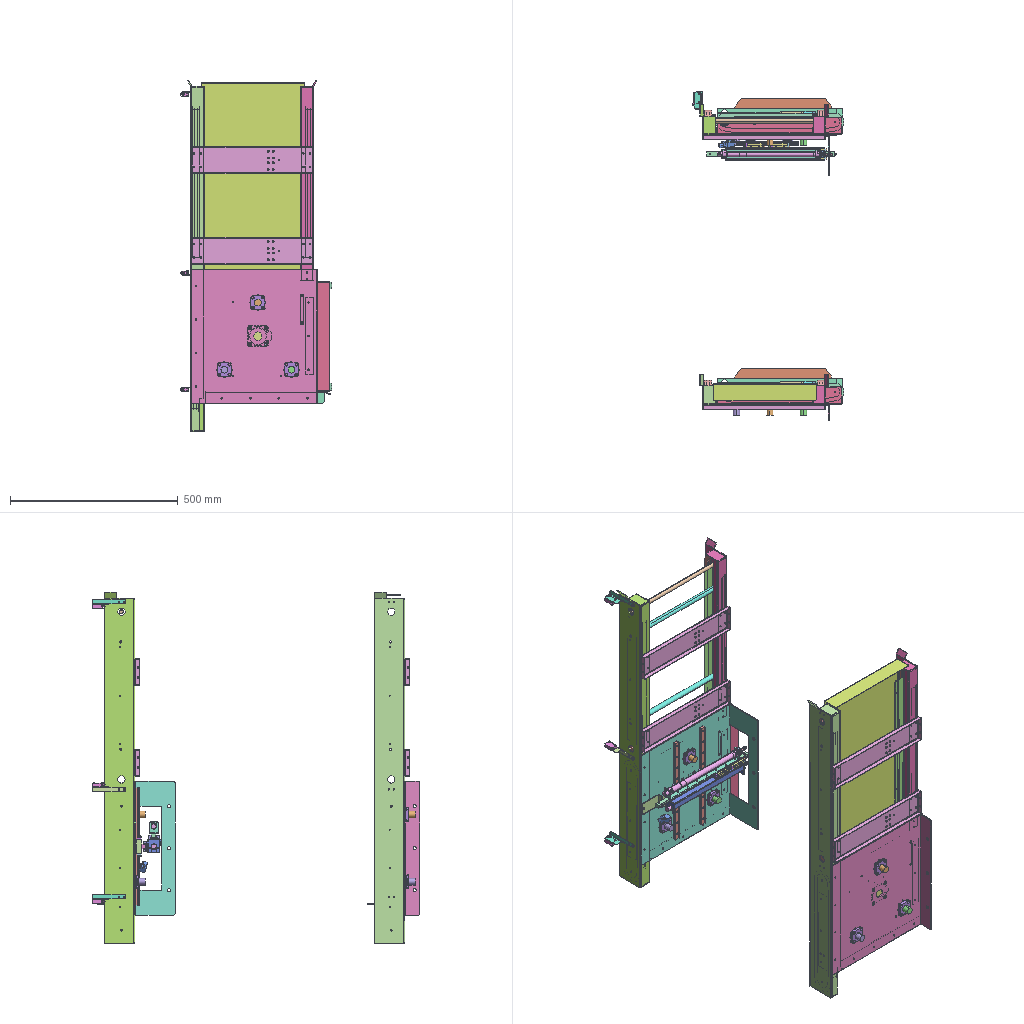Assembly | SolidWorks | 39 different items | 94 placed | box 453 x 977 x 1048 mm
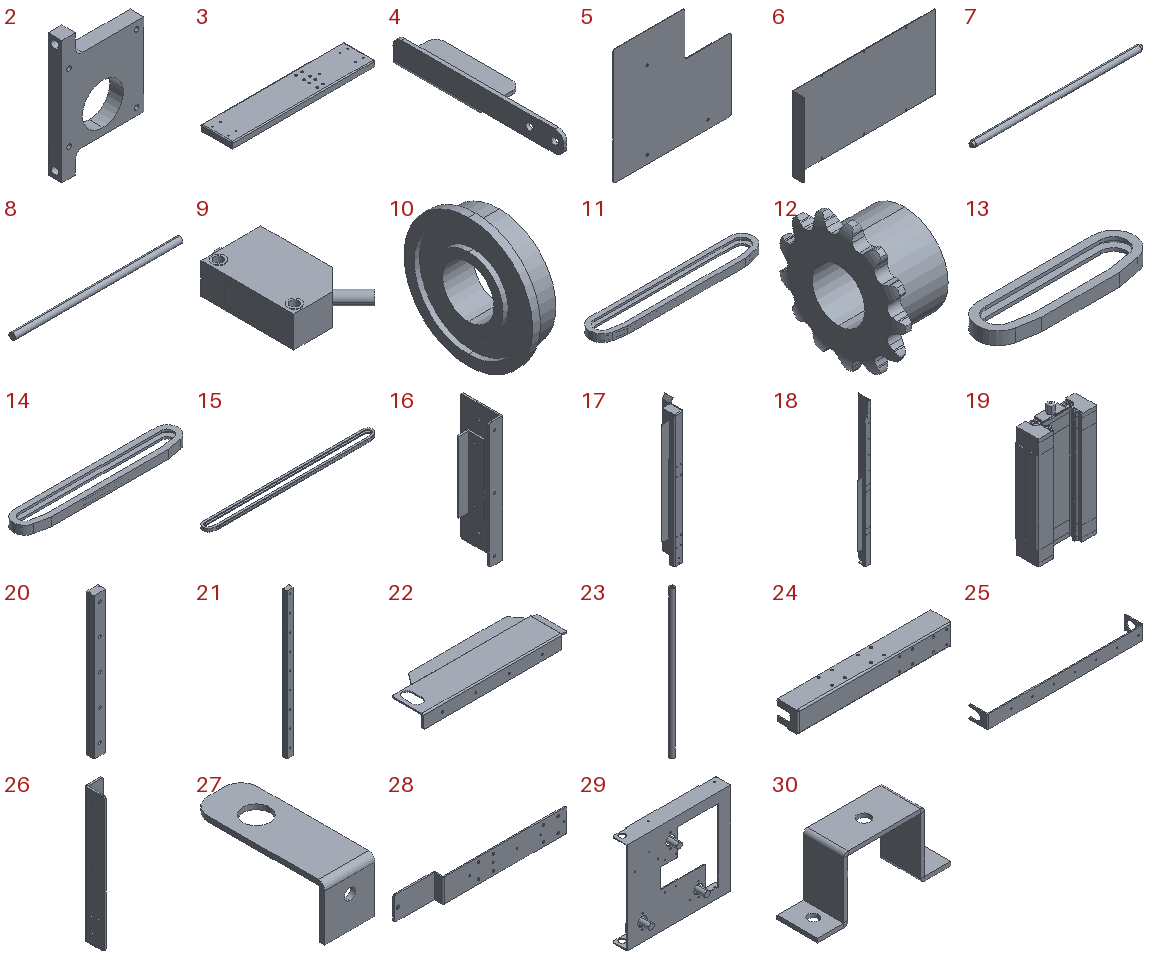Parts list (item | name | quantity | size | volume | features):
1 | 3060 Aluminium Profile3 | x1 | - | - | -
2 | - | x4 | 60 x 10 x 90 mm | 31044 mm3 | features HoleWzd 3, Cut 1, Extrusion 1, Fillet 1, ICE 1, MoveFace 1
3 | - | x4 | 366 x 80 x 15 mm | 79720 mm3 | features HoleWzd 4, EdgeFlange 2, MirrorPattern 2, FlatPattern 1, ICE 1, SMBaseFlange 1, SheetMetal 1
4 | - | x3 | 25 x 100 x 15 mm | 4826 mm3 | features HoleWzd 2, DeleteBody 1, EdgeFlange 1, Fillet 1, FlatPattern 1, MirrorSolid 1, SMBaseFlange 1, SheetMetal 1
5 | - | x2 | 280 x 1.5 x 277 mm | 98876 mm3 | features HoleWzd 2, Fillet 1, FlatPattern 1, ICE 1, SMBaseFlange 1, SheetMetal 1
6 | - | x2 | 595 x 50 x 308 mm | 296830 mm3 | features ICE 2, BreakCorner 1, EdgeFlange 1, Fillet 1, FlatPattern 1, SMBaseFlange 1, SheetMetal 1
7 | - | x1 | 367 x 13 x 13 mm | 48171 mm3 | features ICE 4, Chamfer 1, Extrusion 1, Helix 1, SweepCut 1
8 | - | x2 | 340 x 13 x 13 mm | 45129 mm3 | features Extrusion 1
9 | - | x3 | 24.985 x 38.085 x 10.8 mm | 6244 mm3 | features BaseBody 1
10 | - | x4 | 6 x 25 x 25 mm | 1569 mm3 | features Stock 1
11 | - | x2 | 435 x 70.699 x 20 mm | 118324 mm3 | features Extrusion 1, ICE 1
12 | - | x1 | 15 x 28.727 x 28.922 mm | 3598 mm3 | features ICE 3, CirPattern 1, Cut 1, RefAxis 1, Revolution 1
13 | - | x2 | 245 x 70.699 x 20 mm | 68924 mm3 | features Extrusion 1, ICE 1
14 | - | x4 | 382 x 57.598 x 20 mm | 102612 mm3 | features Extrusion 1, ICE 1
15 | - | x4 | 1035 x 70.699 x 20 mm | 274324 mm3 | features Extrusion 1, ICE 1
16 | - | x2 | 25 x 75 x 230 mm | 84822 mm3 | features HoleWzd 4, Fillet 2, FlattenBends 2, ProcessBends 2, BossThin 1, ExtruThin 1
17 | - | x2 | 49.598 x 90 x 598.124 mm | 346794 mm3 | features HoleWzd 12, EdgeFlange 6, Fillet 2, FlatPattern 2, ICE 2, SMBaseFlange 2, SheetMetal 2
18 | - | x2 | 49.598 x 90 x 1048 mm | 529976 mm3 | features HoleWzd 13, EdgeFlange 6, ICE 4, Fillet 2, FlatPattern 2, SMBaseFlange 2, SheetMetal 2
19 | - | x6 | 32 x 12 x 63.373 mm | 16736 mm3 | features ICE 21, MirrorSolid 4, Extrusion 3, Fillet 3, MirrorPattern 3, RevCut 3, Chamfer 2, Dome 2, DeleteBody 1, LPattern 1, LibraryFeature 1
20 | - | x1 | 15 x 10 x 185 mm | 26054 mm3 | features ICE 18, MirrorSolid 4, Extrusion 3, Fillet 3, MirrorPattern 3, RevCut 3, Chamfer 2, Dome 2, DeleteBody 1, LPattern 1, LibraryFeature 1, MoveFace 1
21 | - | x3 | 15 x 10 x 350 mm | 49374 mm3 | features ICE 18, MirrorSolid 4, Extrusion 3, Fillet 3, MirrorPattern 3, RevCut 3, Chamfer 2, Dome 2, DeleteBody 1, LPattern 1, LibraryFeature 1
22 | - | x2 | 374.323 x 110 x 35 mm | 143786 mm3 | features Fillet 3, ICE 3, EdgeFlange 1, ExtruThin 1, FlatPattern 1, FlattenBends 1, HoleWzd 1, ProcessBends 1, SheetMetal 1
23 | - | x1 | 10 x 10 x 321 mm | 24603 mm3 | features HoleWzd 2, Extrusion 1
24 | - | x1 | 295 x 40 x 40 mm | 59293 mm3 | features HoleWzd 3, EdgeFlange 2, ICE 2, FlatPattern 1, MoveFace 1, SMBaseFlange 1, SheetMetal 1
25 | - | x1 | 295 x 35 x 25 mm | 16784 mm3 | features HoleWzd 2, ICE 2, EdgeFlange 1, Fillet 1, FlatPattern 1, LPattern 1, SMBaseFlange 1, SheetMetal 1
26 | - | x2 | 35 x 40 x 270 mm | 57353 mm3 | features HoleWzd 2, Fillet 1, FlatPattern 1, SMBaseFlange 1, SheetMetal 1
27 | - | x1 | 15 x 40 x 16 mm | 1110 mm3 | features EdgeFlange 2, Fillet 2, FlatPattern 1, HoleWzd 1, ICE 1, SMBaseFlange 1, SheetMetal 1
28 | - | x1 | 278 x 17 x 40 mm | 23031 mm3 | features EdgeFlange 2, HoleWzd 2, Fillet 1, FlatPattern 1, ICE 1, LPattern 1, SMBaseFlange 1, SheetMetal 1
29 | - | x2 | 370 x 87 x 328 mm | 480220 mm3 | features HoleWzd 7, ICE 7, Cut 2, Fillet 2, Extrusion 1, FlattenBends 1, MirrorPattern 1, MoveFace 1, ProcessBends 1
30 | - | x6 | 66 x 20 x 32 mm | 4819 mm3 | features EdgeFlange 2, FlatPattern 1, HoleWzd 1, ICE 1, SMBaseFlange 1, SheetMetal 1
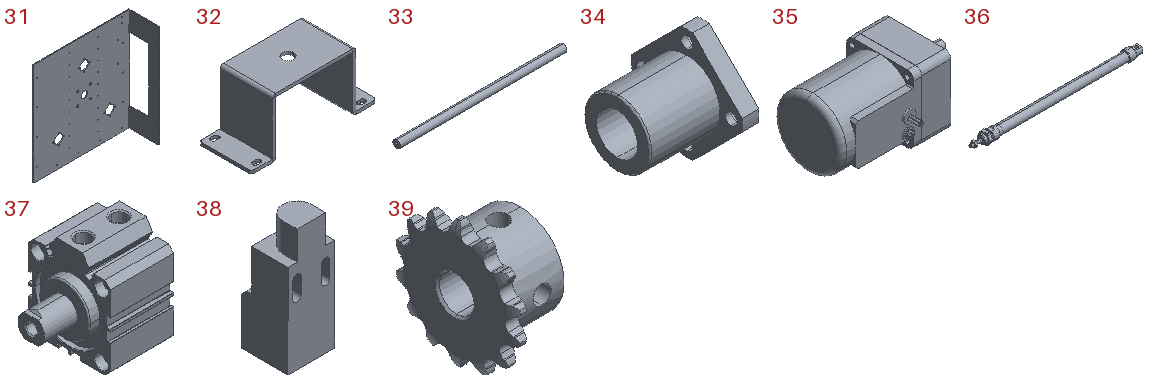31 | - | x2 | 377.5 x 120 x 400 mm | 523953 mm3 | features HoleWzd 10, ICE 3, FlattenBends 2, MoveFace 2, ProcessBends 2, BossThin 1, Extrusion 1, Fillet 1, LPattern 1
32 | - | x2 | 120 x 50 x 56 mm | 32764 mm3 | features EdgeFlange 3, ICE 2, Fillet 1, FlatPattern 1, SMBaseFlange 1, SheetMetal 1
33 | - | x2 | 354 x 16 x 16 mm | 70567 mm3 | features HoleWzd 2, Revolution 1
34 | - | x6 | 42 x 54 x 54 mm | 26429 mm3 | features ICE 8, LPattern 1, LockFeature 1, Revolution 1
35 | - | x4 | 130 x 72 x 60 mm | 275095 mm3 | features BaseBody 2
36 | - | x2 | 344 x 25 x 22 mm | 44525 mm3 | features BaseBody 4, MoveCopyBody 2, CombineBodies 1, MoveFace 1, Split 1
37 | - | x2 | 77 x 62 x 71.5 mm | 138167 mm3 | features BaseBody 2, MoveCopyBody 1
38 | - | x1 | 18 x 18 x 47 mm | 10909 mm3 | features ICE 3, Extrusion 1
39 | - | x1 | 15 x 28.455 x 29 mm | 4351 mm3 | features ICE 3, CirPattern 2, Chamfer 1, Cut 1, HoleWzd 1, RefAxis 1, Revolution 1
Mates (type | each side: item.copy, entity, surface, feature):
Concentric | 18.1 face cylinder Cut-Extrude1 | 15.1 face cylinder Boss-Extrude1
Coincident | 18.1 face plane Base-Flange2 | 15.1 face plane Boss-Extrude1
Coincident | 18.1 face plane Edge-Flange1 | 3.1 face plane Base-Flange1
Coincident | 3.2 face plane Edge-Flange2 | 3.1 face plane Edge-Flange2 | 2 times
Parallel | 31.1 face plane Boss-Extrude1 | 29.1 face plane Boss-Extrude1
Concentric | 31.1 face cylinder Cut-Extrude1 | 37.1 face cylinder SDA-50x2020_r-1-solid1
Concentric | 29.1 face cylinder Cut-Extrude2 | 8.1 face cylinder Boss-Extrude1
Coincident | 31.1 face plane Boss-Extrude1 | 37.1 face plane SDA-50x2020_b-1-solid1
Coincident | 29.1 face plane Boss-Extrude1 | 32.1 face plane Edge-Flange3
Concentric | 32.1 face cylinder Cut-Extrude1 | 37.1 face cylinder SDA-50x2020_r-1-solid1
Parallel | 32.1 face plane Base-Flange1 | 37.1 face plane SDA-50x2020_b-1-solid1
Coincident | 32.1 face plane Base-Flange1 | 37.1 face plane SDA-50x2020_r-1-solid1
Concentric | 14.1 face cylinder Boss-Extrude1 | 8.1 face cylinder Boss-Extrude1
Concentric | 14.1 face cylinder Boss-Extrude1 | 29.1 face cylinder Cut-Extrude2
Coincident | 18.1 face plane Edge-Flange1 | 31.1 face plane Boss-Extrude1
Coincident | 18.1 face plane Base-Flange1 | 31.1 face plane Boss-Extrude1
DistanceDim | 8.1 face plane Boss-Extrude1 | 29.1 face plane Boss-Extrude1
Coincident | 29.1 face plane Mirror1 | 14.1 face plane Boss-Extrude1
Concentric | 8.1 face cylinder Boss-Extrude1 | 14.2 face cylinder Boss-Extrude1
Concentric | 14.1 face cylinder Boss-Extrude1 | 14.2 edge
Coincident | 29.1 face plane Boss-Extrude2 | 14.2 face plane Boss-Extrude1
Coincident | 29.1 face plane Boss-Extrude1 | 35.1 face plane MX6G5BA-1-solid1
Parallel | 29.1 face plane Mirror1 | 35.1 face plane MX6G5BA-1-solid1
DistanceDim | 35.1 face plane MX6G5BA-1-solid1 | 29.1 face plane Mirror1
Coincident | 15.2 face plane Boss-Extrude1 | 13.1 face plane Boss-Extrude1 | 2 times
Concentric | 13.1 face cylinder Boss-Extrude1 | 35.2 face cylinder MX6G5BA-1-solid1
Parallel | 31.1 face plane Boss-Extrude1 | 35.2 face plane MX6G5BA-1-solid1
Concentric | 31.1 face cylinder Cut-Extrude2 | 34.1 face cylinder Revolve1
Concentric | 31.1 face cylinder Cut-Extrude2 | 34.2 face cylinder Revolve1
Concentric | 31.1 face cylinder Cut-Extrude2 | 34.3 face cylinder Revolve1
DistanceDim | 35.1 face plane MX6G5BA-1-solid1 | 29.1 face plane Boss-Extrude1
Coincident | 31.1 face plane Boss-Extrude1 | 34.1 face plane Boss-Extrude1
Coincident | 31.1 face plane Boss-Extrude1 | 34.3 face plane Boss-Extrude1
Coincident | 31.1 face plane Boss-Extrude1 | 34.2 face plane Boss-Extrude1
Concentric | 29.1 face cylinder Boss-Extrude4 | 34.3 face cylinder Revolve1
Concentric | 29.1 face cylinder Boss-Extrude4 | 34.1 face cylinder Revolve1
Coincident | 29.1 face plane Boss-Extrude4 | 30.1 face plane Base-Flange1
Concentric | 29.1 face cylinder M6 Tapped Hole1 | 30.1 face cylinder Cut-Extrude1
Concentric | 29.1 face cylinder Ø4.2 (4.2) Diameter Hole1 | 30.1 face cylinder Ø5.2 (5.2) Diameter Hole1
Coincident | 29.1 face plane Boss-Extrude4 | 30.2 face plane Base-Flange1
Concentric | 29.1 face cylinder M6 Tapped Hole1 | 30.2 face cylinder Cut-Extrude1
Concentric | 29.1 face cylinder Ø4.2 (4.2) Diameter Hole1 | 30.2 face cylinder Ø5.2 (5.2) Diameter Hole1
Coincident | 29.1 face plane Boss-Extrude4 | 30.3 face plane Base-Flange1
Concentric | 29.1 face cylinder M6 Tapped Hole1 | 30.3 face cylinder Cut-Extrude1
Concentric | 29.1 face cylinder Ø4.2 (4.2) Diameter Hole1 | 30.3 face cylinder Ø5.2 (5.2) Diameter Hole1
Concentric | 36.1 face cylinder 16MA 200 Body-1-solid1 | 25.1 face cylinder Cut-Extrude2
Coincident | 36.1 face plane 16MA 200 Body-1-solid1 | 25.1 face plane Edge-Flange2
Concentric | 19.1 face cylinder Mirror17 | 21.1 face cylinder Boss-Extrude11
Concentric | 19.1 face cylinder Cut-Extrude11 | 21.1 face cylinder Boss-Extrude11
Coincident | 25.1 face plane Base-Flange1 | 21.1 face plane Boss-Extrude11
Concentric | 25.1 face cylinder M3 Tapped Hole1 | 21.1 face cylinder LPattern1
DistanceDim | 6.1 face plane Base-Flange1 | 15.2 face plane Boss-Extrude1
Coincident | 21.1 face plane Boss-Extrude11 | 36.2 face plane 16 MA Nut1-1-solid1
Coincident | 31.1 face plane Boss-Extrude1 | 21.2 face plane Boss-Extrude11
Concentric | 19.2 face cylinder Cut-Extrude11 | 21.2 face cylinder Boss-Extrude11 | 2 times
Concentric | 19.3 face cylinder Cut-Extrude11 | 21.3 face cylinder Boss-Extrude11 | 2 times
Coincident | 31.1 face plane Boss-Extrude1 | 21.3 face plane Boss-Extrude11
Coincident | 21.2 face plane Boss-Extrude11 | 21.3 face plane Boss-Extrude11
Coincident | 19.2 face plane Mirror17 | 19.3 face plane Mirror17
DistanceDim | 21.2 face plane Boss-Extrude11 | 21.3 face plane Boss-Extrude11
Concentric | 36.2 face cylinder 16MA 200 Body-1-solid1 | 24.1 face cylinder Cut-Extrude2
Concentric | 21.1 face cylinder Boss-Extrude11 | 19.4 face cylinder Cut-Extrude11 | 2 times
Coincident | 19.4 face plane Boss-Extrude1 | 24.1 face plane Base-Flange1
Coincident | 36.2 face plane 16MA 200 Body-1-solid1 | 24.1 face plane Edge-Flange2
Concentric | 19.1 face cylinder Mirror2 | 24.1 face cylinder Ø4.2 (4.2) Diameter Hole1
Concentric | 19.4 face cylinder Mirror2 | 24.1 face cylinder Ø4.2 (4.2) Diameter Hole1
Coincident | 19.2 face plane Boss-Extrude1 | 28.1 face plane Base-Flange1
Concentric | 19.3 face cylinder Cut-Revolve1 | 28.1 face cylinder Ø4.2 (4.2) Diameter Hole1
Concentric | 19.3 face cylinder Mirror2 | 28.1 face cylinder Ø4.2 (4.2) Diameter Hole1
Coincident | 28.1 face plane Base-Flange1 | 20.1 face plane Boss-Extrude11
Concentric | 28.1 face cylinder M3 Tapped Hole1 | 20.1 face cylinder Cut-Revolve2
Concentric | 28.1 face cylinder LPattern1 | 20.1 face cylinder LPattern1
Concentric | 20.1 face cylinder Boss-Extrude11 | 19.5 face cylinder Cut-Extrude11
Coincident | 20.1 face plane Boss-Extrude11 | 19.5 face plane Cut-Extrude11
Coincident | 20.1 face plane Boss-Extrude11 | 19.6 face plane Cut-Extrude11
Concentric | 20.1 face cylinder Boss-Extrude11 | 19.6 face cylinder Cut-Extrude11
Coincident | 24.1 face plane Edge-Flange1 | 19.6 face plane Boss-Extrude1
Concentric | 24.1 face cylinder Ø4.2 (4.2) Diameter Hole2 | 19.6 face cylinder Mirror2
Concentric | 24.1 face cylinder Ø4.2 (4.2) Diameter Hole2 | 19.5 face cylinder Mirror2
Coincident | 31.1 face plane Boss-Extrude1 | 16.1 face plane Extrude-Thin1
Concentric | 29.1 face cylinder Cut-Extrude2 | 10.1 face cylinder F6900Z Bearing
Coincident | 29.1 face plane Boss-Extrude1 | 10.1 face plane F6900Z Bearing
Concentric | 29.1 face cylinder Cut-Extrude2 | 10.2 face cylinder F6900Z Bearing
Coincident | 29.1 face plane Boss-Extrude2 | 10.2 face plane F6900Z Bearing
Concentric | 35.1 face cylinder MX6G5BA-1-solid1 | 2.1 face cylinder Cut-Extrude3
Parallel | 35.1 face plane MX6G5BA-1-solid1 | 2.1 face plane Boss-Extrude1
Coincident | 35.1 face plane MX6G5BA-1-solid1 | 2.1 face plane Boss-Extrude1
Concentric | 35.2 face cylinder MX6G5BA-1-solid1 | 2.2 face cylinder Cut-Extrude3
Parallel | 35.2 face plane MX6G5BA-1-solid1 | 2.2 face plane Boss-Extrude1
Coincident | 35.2 face plane MX6G5BA-1-solid1 | 2.2 face plane Boss-Extrude1
Width | 29.1 face plane Boss-Extrude1 | 29.1 face plane Boss-Extrude1 | 16.1 face plane Extrude-Thin1 | 16.1 face plane Extrude-Thin1
Coincident | 31.1 face plane Boss-Extrude1 | 22.1 face plane Extrude-Thin1 | 2 times
DistanceDim | 31.1 face plane Extrude-Thin1 | 22.1 face plane Extrude-Thin1
Coincident | 18.1 face plane Edge-Flange1 | 17.1 face plane Edge-Flange1
Coincident | 18.1 face plane Edge-Flange6 | 17.1 face plane Edge-Flange5
DistanceDim | 17.1 face plane Base-Flange1 | 18.1 face plane Base-Flange1
Concentric | 18.1 face cylinder Cut-Extrude2 | 15.1 face cylinder Boss-Extrude1
Coincident | 18.1 face plane Base-Flange1 | 3.2 face plane Edge-Flange2
Coincident | 18.1 face plane Edge-Flange1 | 3.2 face plane Base-Flange1
DistanceDim | 18.1 face plane Edge-Flange6 | 31.1 face plane Boss-Extrude1
Concentric | 18.1 face cylinder Ø3.2 (3.2) Diameter Hole1 | 26.1 face cylinder Ø4.2 (4.2) Diameter Hole1 | 2 times
Coincident | 18.1 face plane Base-Flange1 | 26.1 face plane Base-Flange1
Concentric | 35.1 face cylinder MX6G5BA-1-solid1 | 39.1 face cylinder Revolve
Concentric | 8.1 face cylinder Boss-Extrude1 | 12.1 face cylinder Revolve
Coincident | 12.1 face plane Revolve | 39.1 face plane Revolve
Coincident | 29.1 face plane Boss-Extrude2 | 23.1 face plane Boss-Extrude1
Concentric | 29.1 face cylinder Ø5.2 (5.2) Diameter Hole1 | 23.1 face cylinder Boss-Extrude1
Coincident | 2.1 face plane Boss-Extrude1 | 5.1 face plane Base-Flange1
Concentric | 29.1 face cylinder Cut-Extrude8 | 5.1 face cylinder Ø5.5 (5.5) Diameter Hole1 | 2 times
Concentric | 18.1 face cylinder Ø5.0 (5) Diameter Hole1 | 11.1 face cylinder Boss-Extrude1
Coincident | 18.1 face plane Base-Flange1 | 11.1 face plane Boss-Extrude1
Concentric | 18.1 face cylinder Cut-Extrude1 | 11.1 face cylinder Boss-Extrude1
Concentric | 31.1 face cylinder M3 Tapped Hole1 | 21.2 face cylinder Cut-Revolve2
Parallel | 31.1 face plane Boss-Extrude1 | 21.2 face plane Boss-Extrude11
Coincident | 18.1 face plane Base-Flange1 | 4.1 face plane Edge-Flange1
Coincident | 4.1 face plane Base-Flange1 | 9.1 face plane Imported1
Concentric | 4.1 face cylinder Ø4.0 (4) Diameter Hole1 | 9.1 face cylinder Imported1 | 2 times
Parallel | 18.1 face plane Base-Flange1 | 4.1 face plane Base-Flange1
Coincident | 18.1 face plane Base-Flange1 | 4.2 face plane Mirror1
Parallel | 18.1 face plane Base-Flange1 | 4.2 face plane Mirror1
Coincident | 4.2 face plane Mirror1 | 9.2 face plane Imported1
Concentric | 4.2 face cylinder Mirror1 | 9.2 face cylinder Imported1 | 2 times
Concentric | 18.1 face cylinder Ø3.2 (3.2) Diameter Hole2 | 4.2 face cylinder Mirror1 | 2 times
Concentric | 18.1 face cylinder Ø3.2 (3.2) Diameter Hole2 | 4.1 face cylinder Ø4.2 (4.2) Diameter Hole1 | 2 times
Coincident | 4.3 face plane Mirror1 | 9.3 face plane Imported1
Concentric | 4.3 face cylinder Mirror1 | 9.3 face cylinder Imported1 | 2 times
Coincident | 18.1 face plane Base-Flange1 | 4.3 face plane Mirror1
Parallel | 18.1 face plane Base-Flange1 | 4.3 face plane Mirror1
Concentric | 18.1 face cylinder Ø3.2 (3.2) Diameter Hole2 | 4.3 face cylinder Mirror1 | 2 times
Concentric | 33.1 face cylinder Revolve1 | 17.1 face cylinder Ø6.5 (6.5) Diameter Hole1
Coincident | 33.1 face plane Revolve1 | 17.1 face plane Base-Flange2
Concentric | 33.2 face cylinder Revolve1 | 17.1 face cylinder Ø6.5 (6.5) Diameter Hole1
Coincident | 33.2 face plane Revolve1 | 17.1 face plane Base-Flange2
DistanceDim | 7.1 face plane Boss-Extrude1 | 17.1 face plane Base-Flange1
Concentric | 17.1 edge | 7.1 face cylinder Boss-Extrude1
Parallel | 18.1 face plane Base-Flange1 | 34.3 face plane Cut-Extrude2
Coincident | 36.2 face plane 16MA 200 Body-1-solid1 | 27.1 face plane Base-Flange1
Coincident | 21.1 face plane Boss-Extrude11 | 27.1 face plane Edge-Flange1 | 2 times
DistanceDim | 24.1 face plane Edge-Flange2 | 31.1 face plane Extrude-Thin1
DistanceDim | 2.2 face plane Boss-Extrude1 | 31.1 face plane Extrude-Thin1
DistanceDim | 2.2 face plane Boss-Extrude1 | 31.1 face plane Boss-Extrude1
Concentric | 25.1 face cylinder LPattern1 | 21.1 face cylinder LPattern1